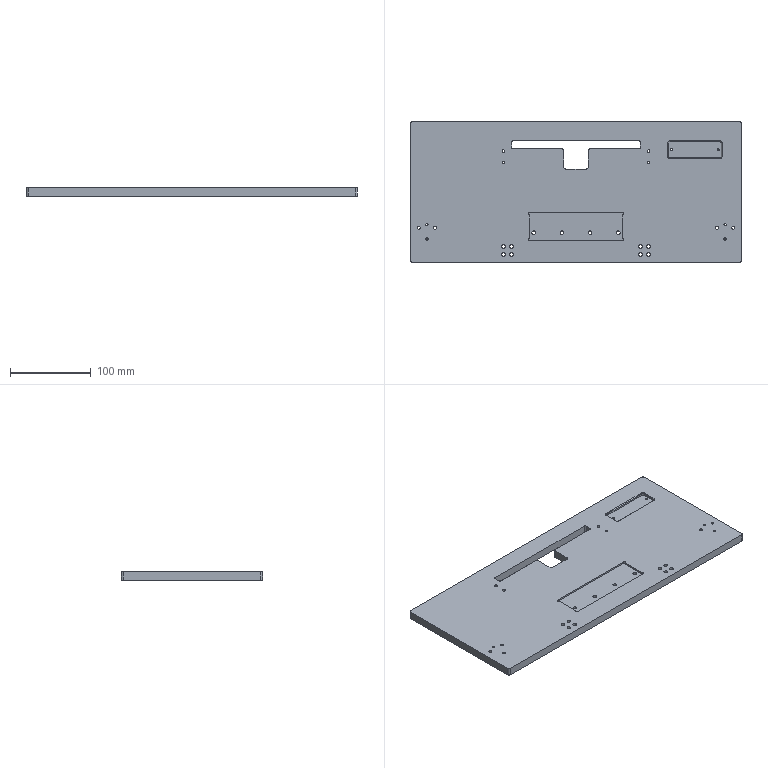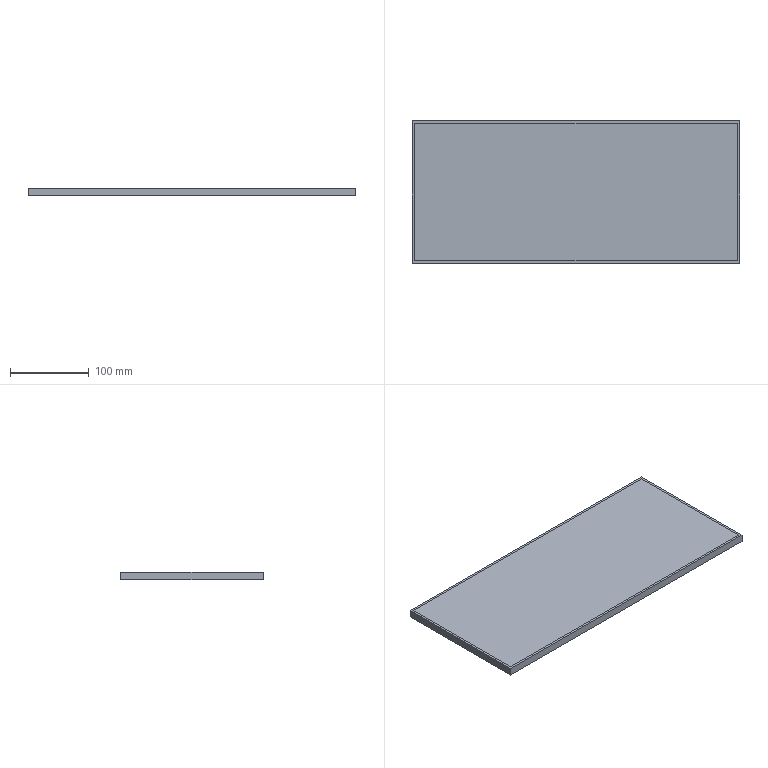CAM job | NX | 3-axis milling, drilling | part box 410 x 175 x 10 mm | stock box 416 x 181 x 10 mm
Tools:
number,name,description,diameter,corner_radius,flute_length,length,flutes
2,D4A45,Milling Tool-5 Parameters,4.0,0.0,2.0,2.0,2
9,D10,Milling Tool-5 Parameters,10.0,0.0,50.0,75.0,2
4,D4,Milling Tool-5 Parameters,4.0,0.0,50.0,75.0,2
3,D3,Milling Tool-5 Parameters,3.0,0.0,50.0,75.0,2
10,D10JING,Milling Tool-5 Parameters,10.0,0.0,50.0,75.0,2
15,3.5ZT,Drilling Tool,3.5,0.0,35.0,50.0,2
13,3.0ZT,Drilling Tool,3.0,0.0,35.0,50.0,2
11,2.5ZT,Drilling Tool,2.5,0.0,35.0,50.0,2
16,4.5ZT,Drilling Tool,4.5,0.0,35.0,50.0,2
6,D6,Milling Tool-5 Parameters,6.0,0.0,50.0,75.0,2
Operations:
program,operation,operation_type,tool,method,geometry_group,spindle_rpm,surface_speed,feed_per_tooth,feed_cut,feed_plunge,cut_length_mm,path_length_mm,cut_time_min,machine_time_min
1吸,ZLEVEL_PROFILE_1_COPY_1_COPY,ZLevelMilling,D4A45,METHOD,A,9500.0,179.0,0.0526,1000.0,100.0,2147.303,5665.83,2.147,2.499
1吸,DRILLING,Operation,D4A45,METHOD,A,5000.0,62.0,0.025,250.0,0.0,104.0,1171.808,0.416,0.5228
1吸,ZLEVEL_PROFILE,ZLevelMilling,D10,METHOD,A,9500.0,298.0,0.1579,3000.0,1000.0,12090.449,12157.149,4.062,4.068
1吸,CAVITY_MILL,CavityMilling,D10,METHOD,A,9500.0,298.0,0.1579,3000.0,1000.0,4162.216,4747.202,1.857,1.916
1吸,CAVITY_MILL_COPY,CavityMilling,D4,METHOD,A,9500.0,119.0,0.1053,2000.0,1000.0,12468.69,14173.142,6.402,6.573
1吸,FLOOR_WALL,VolumeBased25DMillingOperation,D4,METHOD,A,9500.0,119.0,0.0526,1000.0,100.0,3013.087,3270.2,3.013,3.039
1吸,ZLEVEL_PROFILE_COPY,ZLevelMilling,D4,METHOD,A,9500.0,119.0,0.0632,1200.0,1000.0,375.734,452.434,0.3135,0.3212
1吸,CAVITY_MILL_COPY_COPY,CavityMilling,D3,METHOD,A,9500.0,89.0,0.0684,1300.0,1000.0,115.698,554.949,0.0939,0.1378
1吸,ZLEVEL_PROFILE_COPY_COPY,ZLevelMilling,D10JING,METHOD,A,9500.0,119.0,0.0632,1200.0,1000.0,1206.366,1283.066,1.006,1.014
2虎钳,DRILLING_COPY,Operation,D4A45,METHOD,B,5000.0,62.0,0.025,250.0,0.0,104.0,1191.808,0.416,0.5248
2虎钳,DRILLING_COPY_COPY,Operation,3.5ZT,METHOD,B,1910.0,21.0,0.0471,180.0,0.0,124.412,813.837,0.6912,0.7601
2虎钳,DRILLING_COPY_COPY_COPY,Operation,3.0ZT,METHOD,B,1910.0,21.0,0.0471,180.0,0.0,61.605,598.719,0.3423,0.396
2虎钳,DRILLING_COPY_COPY_COPY_COPY,Operation,2.5ZT,METHOD,B,1910.0,21.0,0.0471,180.0,0.0,24.502,170.082,0.1361,0.1507
2虎钳,DRILLING_COPY_COPY_COPY_1,Operation,4.5ZT,METHOD,B,1910.0,21.0,0.0471,180.0,0.0,184.223,694.412,1.024,1.075
2虎钳,HOLE_MILLING,CylinderMilling,D6,METHOD,B,9500.0,179.0,0.0789,1500.0,100.0,1101.831,2105.491,0.7346,0.8349
2虎钳,ZLEVEL_PROFILE_1_COPY_1_COPY_COPY,ZLevelMilling,D4A45,METHOD,B,9500.0,179.0,0.0526,1000.0,100.0,1958.272,7734.355,1.958,2.536